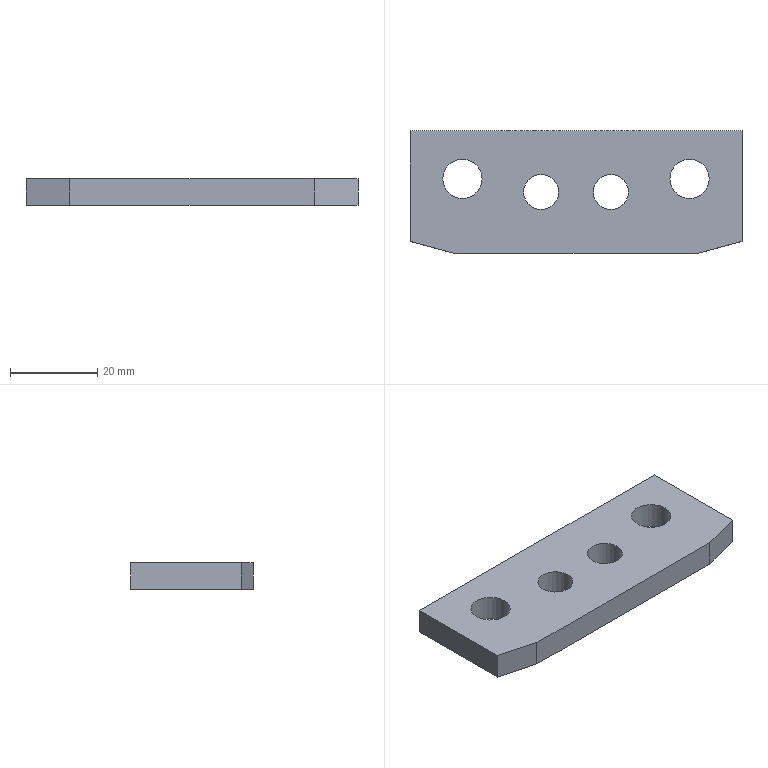Part | STEP file | gslz 2016.10.28-13_id1586_x_t | 1 solid | 12 faces | box 76 x 28 x 6 mm | volume 11241 mm3 | plane 8 | cylinder 4 | commonest cylinder face diameters 8 x2 9 x2
STEP:
#1=CARTESIAN_POINT('',(0.,0.,0.));
#2=DIRECTION('',(0.,0.,1.));
#3=DIRECTION('',(1.,0.,0.));
#4=AXIS2_PLACEMENT_3D('',#1,#2,#3);
#5=CARTESIAN_POINT('',(-1350.002,284.2,6.));
#6=VERTEX_POINT('',#5);
#7=CARTESIAN_POINT('',(-1358.002,284.2,6.));
#8=VERTEX_POINT('',#7);
#9=CARTESIAN_POINT('',(-1354.002,284.2,6.));
#10=DIRECTION('',(0.,0.,1.));
#11=DIRECTION('',(-1.,0.,0.));
#12=AXIS2_PLACEMENT_3D('',#9,#10,#11);
#13=CIRCLE('',#12,4.);
#14=CARTESIAN_POINT('',(-1354.002,284.2,-73.));
#15=DIRECTION('',(0.,0.,1.));
#16=DIRECTION('',(1.,0.,0.));
#17=AXIS2_PLACEMENT_3D('',#14,#15,#16);
#18=CYLINDRICAL_SURFACE('',#17,4.);
#19=CARTESIAN_POINT('',(-3.142,79.));
#20=DIRECTION('',(1.,0.));
#21=VECTOR('',#20,1.);
#22=LINE('',#19,#21);
#23=(GEOMETRIC_REPRESENTATION_CONTEXT(2)PARAMETRIC_REPRESENTATION_CONTEXT()REPRESENTATION_CONTEXT('',''));
#24=DEFINITIONAL_REPRESENTATION('',(#22),#23);
#25=PCURVE('',#18,#24);
#26=CARTESIAN_POINT('',(-1421.002,267.7,6.));
#27=DIRECTION('',(0.,0.,-1.));
#28=DIRECTION('',(-1.,0.,0.));
#29=AXIS2_PLACEMENT_3D('',#26,#27,#28);
#30=PLANE('',#29);
#31=CARTESIAN_POINT('',(-63.,16.5));
#32=CARTESIAN_POINT('',(-63.,9.572));
#33=CARTESIAN_POINT('',(-69.,13.036));
#34=CARTESIAN_POINT('',(-75.,16.5));
#35=CARTESIAN_POINT('',(-69.,19.964));
#36=CARTESIAN_POINT('',(-63.,23.428));
#37=CARTESIAN_POINT('',(-63.,16.5));
#38=(BOUNDED_CURVE()B_SPLINE_CURVE(2,(#31,#32,#33,#34,#35,#36,#37),.UNSPECIFIED.,.T.,.F.)B_SPLINE_CURVE_WITH_KNOTS((1,2,2,2,2,1),(-2.094,0.,2.094,4.189,6.283,8.378),.UNSPECIFIED.)CURVE()GEOMETRIC_REPRESENTATION_ITEM()RATIONAL_B_SPLINE_CURVE((1.,0.5,1.,0.5,1.,0.5,1.))REPRESENTATION_ITEM(''));
#39=(GEOMETRIC_REPRESENTATION_CONTEXT(2)PARAMETRIC_REPRESENTATION_CONTEXT()REPRESENTATION_CONTEXT('',''));
#40=DEFINITIONAL_REPRESENTATION('',(#38),#39);
#41=PCURVE('',#30,#40);
#42=SURFACE_CURVE('',#13,(#25,#41),.PCURVE_S1.);
#43=EDGE_CURVE('',#6,#8,#42,.T.);
#44=ORIENTED_EDGE('',*,*,#43,.F.);
#45=CARTESIAN_POINT('',(-1350.002,284.2,0.));
#46=VERTEX_POINT('',#45);
#47=CARTESIAN_POINT('',(-1350.002,284.2,0.));
#48=CARTESIAN_POINT('',(-1350.002,284.2,6.));
#49=B_SPLINE_CURVE_WITH_KNOTS('',1,(#47,#48),.UNSPECIFIED.,.F.,.F.,(2,2),(73.,79.),.PIECEWISE_BEZIER_KNOTS.);
#50=CARTESIAN_POINT('',(0.,0.));
#51=DIRECTION('',(0.,1.));
#52=VECTOR('',#51,1.);
#53=LINE('',#50,#52);
#54=(GEOMETRIC_REPRESENTATION_CONTEXT(2)PARAMETRIC_REPRESENTATION_CONTEXT()REPRESENTATION_CONTEXT('',''));
#55=DEFINITIONAL_REPRESENTATION('',(#53),#54);
#56=PCURVE('',#18,#55);
#57=CARTESIAN_POINT('',(6.283,0.));
#58=DIRECTION('',(0.,1.));
#59=VECTOR('',#58,1.);
#60=LINE('',#57,#59);
#61=(GEOMETRIC_REPRESENTATION_CONTEXT(2)PARAMETRIC_REPRESENTATION_CONTEXT()REPRESENTATION_CONTEXT('',''));
#62=DEFINITIONAL_REPRESENTATION('',(#60),#61);
#63=PCURVE('',#18,#62);
#64=SEAM_CURVE('',#49,(#56,#63),.PCURVE_S1.);
#65=EDGE_CURVE('',#46,#6,#64,.T.);
#66=ORIENTED_EDGE('',*,*,#65,.F.);
#67=CARTESIAN_POINT('',(-1354.002,284.2,0.));
#68=DIRECTION('',(0.,0.,-1.));
#69=DIRECTION('',(1.,0.,0.));
#70=AXIS2_PLACEMENT_3D('',#67,#68,#69);
#71=CIRCLE('',#70,4.);
#72=CARTESIAN_POINT('',(6.283,73.));
#73=DIRECTION('',(-1.,0.));
#74=VECTOR('',#73,1.);
#75=LINE('',#72,#74);
#76=(GEOMETRIC_REPRESENTATION_CONTEXT(2)PARAMETRIC_REPRESENTATION_CONTEXT()REPRESENTATION_CONTEXT('',''));
#77=DEFINITIONAL_REPRESENTATION('',(#75),#76);
#78=PCURVE('',#18,#77);
#79=CARTESIAN_POINT('',(-1461.002,298.2,0.));
#80=DIRECTION('',(0.,0.,1.));
#81=DIRECTION('',(1.,0.,0.));
#82=AXIS2_PLACEMENT_3D('',#79,#80,#81);
#83=PLANE('',#82);
#84=CARTESIAN_POINT('',(111.,-14.));
#85=CARTESIAN_POINT('',(111.,-20.928));
#86=CARTESIAN_POINT('',(105.,-17.464));
#87=CARTESIAN_POINT('',(99.,-14.));
#88=CARTESIAN_POINT('',(105.,-10.536));
#89=CARTESIAN_POINT('',(111.,-7.072));
#90=CARTESIAN_POINT('',(111.,-14.));
#91=(BOUNDED_CURVE()B_SPLINE_CURVE(2,(#84,#85,#86,#87,#88,#89,#90),.UNSPECIFIED.,.T.,.F.)B_SPLINE_CURVE_WITH_KNOTS((1,2,2,2,2,1),(-2.094,0.,2.094,4.189,6.283,8.378),.UNSPECIFIED.)CURVE()GEOMETRIC_REPRESENTATION_ITEM()RATIONAL_B_SPLINE_CURVE((1.,0.5,1.,0.5,1.,0.5,1.))REPRESENTATION_ITEM(''));
#92=(GEOMETRIC_REPRESENTATION_CONTEXT(2)PARAMETRIC_REPRESENTATION_CONTEXT()REPRESENTATION_CONTEXT('',''));
#93=DEFINITIONAL_REPRESENTATION('',(#91),#92);
#94=PCURVE('',#83,#93);
#95=SURFACE_CURVE('',#71,(#78,#94),.PCURVE_S1.);
#96=EDGE_CURVE('',#46,#46,#95,.T.);
#97=ORIENTED_EDGE('',*,*,#96,.F.);
#98=ORIENTED_EDGE('',*,*,#65,.T.);
#99=CARTESIAN_POINT('',(-1354.002,284.2,6.));
#100=DIRECTION('',(0.,0.,1.));
#101=DIRECTION('',(-1.,0.,0.));
#102=AXIS2_PLACEMENT_3D('',#99,#100,#101);
#103=CIRCLE('',#102,4.);
#104=CARTESIAN_POINT('',(3.142,79.));
#105=DIRECTION('',(1.,0.));
#106=VECTOR('',#105,1.);
#107=LINE('',#104,#106);
#108=(GEOMETRIC_REPRESENTATION_CONTEXT(2)PARAMETRIC_REPRESENTATION_CONTEXT()REPRESENTATION_CONTEXT('',''));
#109=DEFINITIONAL_REPRESENTATION('',(#107),#108);
#110=PCURVE('',#18,#109);
#111=CARTESIAN_POINT('',(-63.,16.5));
#112=CARTESIAN_POINT('',(-63.,9.572));
#113=CARTESIAN_POINT('',(-69.,13.036));
#114=CARTESIAN_POINT('',(-75.,16.5));
#115=CARTESIAN_POINT('',(-69.,19.964));
#116=CARTESIAN_POINT('',(-63.,23.428));
#117=CARTESIAN_POINT('',(-63.,16.5));
#118=(BOUNDED_CURVE()B_SPLINE_CURVE(2,(#111,#112,#113,#114,#115,#116,#117),.UNSPECIFIED.,.T.,.F.)B_SPLINE_CURVE_WITH_KNOTS((1,2,2,2,2,1),(-2.094,0.,2.094,4.189,6.283,8.378),.UNSPECIFIED.)CURVE()GEOMETRIC_REPRESENTATION_ITEM()RATIONAL_B_SPLINE_CURVE((1.,0.5,1.,0.5,1.,0.5,1.))REPRESENTATION_ITEM(''));
#119=(GEOMETRIC_REPRESENTATION_CONTEXT(2)PARAMETRIC_REPRESENTATION_CONTEXT()REPRESENTATION_CONTEXT('',''));
#120=DEFINITIONAL_REPRESENTATION('',(#118),#119);
#121=PCURVE('',#30,#120);
#122=SURFACE_CURVE('',#103,(#110,#121),.PCURVE_S1.);
#123=EDGE_CURVE('',#8,#6,#122,.T.);
#124=ORIENTED_EDGE('',*,*,#123,.F.);
#125=EDGE_LOOP('',(#44,#66,#97,#98,#124));
#126=FACE_BOUND('',#125,.F.);
#127=ADVANCED_FACE('',(#126),#18,.F.);
#128=CARTESIAN_POINT('',(-1342.002,284.2,6.));
#129=VERTEX_POINT('',#128);
#130=CARTESIAN_POINT('',(-1334.002,284.2,6.));
#131=VERTEX_POINT('',#130);
#132=CARTESIAN_POINT('',(-1338.002,284.2,6.));
#133=DIRECTION('',(0.,0.,-1.));
#134=DIRECTION('',(-1.,0.,0.));
#135=AXIS2_PLACEMENT_3D('',#132,#133,#134);
#136=CIRCLE('',#135,4.);
#137=CARTESIAN_POINT('',(-1338.002,284.2,-73.));
#138=DIRECTION('',(0.,0.,1.));
#139=DIRECTION('',(1.,0.,0.));
#140=AXIS2_PLACEMENT_3D('',#137,#138,#139);
#141=CYLINDRICAL_SURFACE('',#140,4.);
#142=CARTESIAN_POINT('',(3.142,79.));
#143=DIRECTION('',(-1.,0.));
#144=VECTOR('',#143,1.);
#145=LINE('',#142,#144);
#146=(GEOMETRIC_REPRESENTATION_CONTEXT(2)PARAMETRIC_REPRESENTATION_CONTEXT()REPRESENTATION_CONTEXT('',''));
#147=DEFINITIONAL_REPRESENTATION('',(#145),#146);
#148=PCURVE('',#141,#147);
#149=CARTESIAN_POINT('',(-83.,16.5));
#150=DIRECTION('',(1.,0.));
#151=AXIS2_PLACEMENT_2D('',#149,#150);
#152=CIRCLE('',#151,4.);
#153=(GEOMETRIC_REPRESENTATION_CONTEXT(2)PARAMETRIC_REPRESENTATION_CONTEXT()REPRESENTATION_CONTEXT('',''));
#154=DEFINITIONAL_REPRESENTATION('',(#152),#153);
#155=PCURVE('',#30,#154);
#156=SURFACE_CURVE('',#136,(#148,#155),.PCURVE_S1.);
#157=EDGE_CURVE('',#129,#131,#156,.T.);
#158=ORIENTED_EDGE('',*,*,#157,.T.);
#159=CARTESIAN_POINT('',(-1334.002,284.2,0.));
#160=VERTEX_POINT('',#159);
#161=CARTESIAN_POINT('',(-1334.002,284.2,0.));
#162=CARTESIAN_POINT('',(-1334.002,284.2,6.));
#163=B_SPLINE_CURVE_WITH_KNOTS('',1,(#161,#162),.UNSPECIFIED.,.F.,.F.,(2,2),(73.,79.),.PIECEWISE_BEZIER_KNOTS.);
#164=CARTESIAN_POINT('',(0.,0.));
#165=DIRECTION('',(0.,1.));
#166=VECTOR('',#165,1.);
#167=LINE('',#164,#166);
#168=(GEOMETRIC_REPRESENTATION_CONTEXT(2)PARAMETRIC_REPRESENTATION_CONTEXT()REPRESENTATION_CONTEXT('',''));
#169=DEFINITIONAL_REPRESENTATION('',(#167),#168);
#170=PCURVE('',#141,#169);
#171=CARTESIAN_POINT('',(6.283,0.));
#172=DIRECTION('',(0.,1.));
#173=VECTOR('',#172,1.);
#174=LINE('',#171,#173);
#175=(GEOMETRIC_REPRESENTATION_CONTEXT(2)PARAMETRIC_REPRESENTATION_CONTEXT()REPRESENTATION_CONTEXT('',''));
#176=DEFINITIONAL_REPRESENTATION('',(#174),#175);
#177=PCURVE('',#141,#176);
#178=SEAM_CURVE('',#163,(#170,#177),.PCURVE_S1.);
#179=EDGE_CURVE('',#160,#131,#178,.T.);
#180=ORIENTED_EDGE('',*,*,#179,.F.);
#181=CARTESIAN_POINT('',(-1338.002,284.2,0.));
#182=DIRECTION('',(0.,0.,1.));
#183=DIRECTION('',(1.,0.,0.));
#184=AXIS2_PLACEMENT_3D('',#181,#182,#183);
#185=CIRCLE('',#184,4.);
#186=CARTESIAN_POINT('',(0.,73.));
#187=DIRECTION('',(1.,0.));
#188=VECTOR('',#187,1.);
#189=LINE('',#186,#188);
#190=(GEOMETRIC_REPRESENTATION_CONTEXT(2)PARAMETRIC_REPRESENTATION_CONTEXT()REPRESENTATION_CONTEXT('',''));
#191=DEFINITIONAL_REPRESENTATION('',(#189),#190);
#192=PCURVE('',#141,#191);
#193=CARTESIAN_POINT('',(123.,-14.));
#194=DIRECTION('',(1.,0.));
#195=AXIS2_PLACEMENT_2D('',#193,#194);
#196=CIRCLE('',#195,4.);
#197=(GEOMETRIC_REPRESENTATION_CONTEXT(2)PARAMETRIC_REPRESENTATION_CONTEXT()REPRESENTATION_CONTEXT('',''));
#198=DEFINITIONAL_REPRESENTATION('',(#196),#197);
#199=PCURVE('',#83,#198);
#200=SURFACE_CURVE('',#185,(#192,#199),.PCURVE_S1.);
#201=EDGE_CURVE('',#160,#160,#200,.T.);
#202=ORIENTED_EDGE('',*,*,#201,.T.);
#203=ORIENTED_EDGE('',*,*,#179,.T.);
#204=CARTESIAN_POINT('',(-1338.002,284.2,6.));
#205=DIRECTION('',(0.,0.,-1.));
#206=DIRECTION('',(-1.,0.,0.));
#207=AXIS2_PLACEMENT_3D('',#204,#205,#206);
#208=CIRCLE('',#207,4.);
#209=CARTESIAN_POINT('',(9.425,79.));
#210=DIRECTION('',(-1.,0.));
#211=VECTOR('',#210,1.);
#212=LINE('',#209,#211);
#213=(GEOMETRIC_REPRESENTATION_CONTEXT(2)PARAMETRIC_REPRESENTATION_CONTEXT()REPRESENTATION_CONTEXT('',''));
#214=DEFINITIONAL_REPRESENTATION('',(#212),#213);
#215=PCURVE('',#141,#214);
#216=CARTESIAN_POINT('',(-83.,16.5));
#217=DIRECTION('',(1.,0.));
#218=AXIS2_PLACEMENT_2D('',#216,#217);
#219=CIRCLE('',#218,4.);
#220=(GEOMETRIC_REPRESENTATION_CONTEXT(2)PARAMETRIC_REPRESENTATION_CONTEXT()REPRESENTATION_CONTEXT('',''));
#221=DEFINITIONAL_REPRESENTATION('',(#219),#220);
#222=PCURVE('',#30,#221);
#223=SURFACE_CURVE('',#208,(#215,#222),.PCURVE_S1.);
#224=EDGE_CURVE('',#131,#129,#223,.T.);
#225=ORIENTED_EDGE('',*,*,#224,.T.);
#226=EDGE_LOOP('',(#158,#180,#202,#203,#225));
#227=FACE_BOUND('',#226,.F.);
#228=ADVANCED_FACE('',(#227),#141,.F.);
#229=CARTESIAN_POINT('',(-1376.502,287.2,6.));
#230=VERTEX_POINT('',#229);
#231=CARTESIAN_POINT('',(-1372.002,287.2,6.));
#232=DIRECTION('',(0.,0.,-1.));
#233=DIRECTION('',(-1.,0.,0.));
#234=AXIS2_PLACEMENT_3D('',#231,#232,#233);
#235=CIRCLE('',#234,4.5);
#236=CARTESIAN_POINT('',(-1372.002,287.2,47.));
#237=DIRECTION('',(0.,0.,-1.));
#238=DIRECTION('',(-1.,0.,0.));
#239=AXIS2_PLACEMENT_3D('',#236,#237,#238);
#240=CYLINDRICAL_SURFACE('',#239,4.5);
#241=CARTESIAN_POINT('',(0.,41.));
#242=DIRECTION('',(1.,0.));
#243=VECTOR('',#242,1.);
#244=LINE('',#241,#243);
#245=(GEOMETRIC_REPRESENTATION_CONTEXT(2)PARAMETRIC_REPRESENTATION_CONTEXT()REPRESENTATION_CONTEXT('',''));
#246=DEFINITIONAL_REPRESENTATION('',(#244),#245);
#247=PCURVE('',#240,#246);
#248=CARTESIAN_POINT('',(-49.,19.5));
#249=DIRECTION('',(1.,0.));
#250=AXIS2_PLACEMENT_2D('',#248,#249);
#251=CIRCLE('',#250,4.5);
#252=(GEOMETRIC_REPRESENTATION_CONTEXT(2)PARAMETRIC_REPRESENTATION_CONTEXT()REPRESENTATION_CONTEXT('',''));
#253=DEFINITIONAL_REPRESENTATION('',(#251),#252);
#254=PCURVE('',#30,#253);
#255=SURFACE_CURVE('',#235,(#247,#254),.PCURVE_S1.);
#256=EDGE_CURVE('',#230,#230,#255,.T.);
#257=ORIENTED_EDGE('',*,*,#256,.T.);
#258=CARTESIAN_POINT('',(-1376.502,287.2,0.));
#259=VERTEX_POINT('',#258);
#260=CARTESIAN_POINT('',(-1376.502,287.2,6.));
#261=CARTESIAN_POINT('',(-1376.502,287.2,0.));
#262=B_SPLINE_CURVE_WITH_KNOTS('',1,(#260,#261),.UNSPECIFIED.,.F.,.F.,(2,2),(41.,47.),.PIECEWISE_BEZIER_KNOTS.);
#263=CARTESIAN_POINT('',(6.283,0.));
#264=DIRECTION('',(0.,1.));
#265=VECTOR('',#264,1.);
#266=LINE('',#263,#265);
#267=(GEOMETRIC_REPRESENTATION_CONTEXT(2)PARAMETRIC_REPRESENTATION_CONTEXT()REPRESENTATION_CONTEXT('',''));
#268=DEFINITIONAL_REPRESENTATION('',(#266),#267);
#269=PCURVE('',#240,#268);
#270=CARTESIAN_POINT('',(0.,0.));
#271=DIRECTION('',(0.,1.));
#272=VECTOR('',#271,1.);
#273=LINE('',#270,#272);
#274=(GEOMETRIC_REPRESENTATION_CONTEXT(2)PARAMETRIC_REPRESENTATION_CONTEXT()REPRESENTATION_CONTEXT('',''));
#275=DEFINITIONAL_REPRESENTATION('',(#273),#274);
#276=PCURVE('',#240,#275);
#277=SEAM_CURVE('',#262,(#269,#276),.PCURVE_S1.);
#278=EDGE_CURVE('',#230,#259,#277,.T.);
#279=ORIENTED_EDGE('',*,*,#278,.T.);
#280=CARTESIAN_POINT('',(-1367.502,287.2,0.));
#281=VERTEX_POINT('',#280);
#282=CARTESIAN_POINT('',(-1372.002,287.2,0.));
#283=DIRECTION('',(0.,0.,1.));
#284=DIRECTION('',(1.,0.,0.));
#285=AXIS2_PLACEMENT_3D('',#282,#283,#284);
#286=CIRCLE('',#285,4.5);
#287=CARTESIAN_POINT('',(9.425,47.));
#288=DIRECTION('',(-1.,0.));
#289=VECTOR('',#288,1.);
#290=LINE('',#287,#289);
#291=(GEOMETRIC_REPRESENTATION_CONTEXT(2)PARAMETRIC_REPRESENTATION_CONTEXT()REPRESENTATION_CONTEXT('',''));
#292=DEFINITIONAL_REPRESENTATION('',(#290),#291);
#293=PCURVE('',#240,#292);
#294=CARTESIAN_POINT('',(89.,-11.));
#295=DIRECTION('',(1.,0.));
#296=AXIS2_PLACEMENT_2D('',#294,#295);
#297=CIRCLE('',#296,4.5);
#298=(GEOMETRIC_REPRESENTATION_CONTEXT(2)PARAMETRIC_REPRESENTATION_CONTEXT()REPRESENTATION_CONTEXT('',''));
#299=DEFINITIONAL_REPRESENTATION('',(#297),#298);
#300=PCURVE('',#83,#299);
#301=SURFACE_CURVE('',#286,(#293,#300),.PCURVE_S1.);
#302=EDGE_CURVE('',#259,#281,#301,.T.);
#303=ORIENTED_EDGE('',*,*,#302,.T.);
#304=CARTESIAN_POINT('',(-1372.002,287.2,0.));
#305=DIRECTION('',(0.,0.,1.));
#306=DIRECTION('',(1.,0.,0.));
#307=AXIS2_PLACEMENT_3D('',#304,#305,#306);
#308=CIRCLE('',#307,4.5);
#309=CARTESIAN_POINT('',(3.142,47.));
#310=DIRECTION('',(-1.,0.));
#311=VECTOR('',#310,1.);
#312=LINE('',#309,#311);
#313=(GEOMETRIC_REPRESENTATION_CONTEXT(2)PARAMETRIC_REPRESENTATION_CONTEXT()REPRESENTATION_CONTEXT('',''));
#314=DEFINITIONAL_REPRESENTATION('',(#312),#313);
#315=PCURVE('',#240,#314);
#316=CARTESIAN_POINT('',(89.,-11.));
#317=DIRECTION('',(1.,0.));
#318=AXIS2_PLACEMENT_2D('',#316,#317);
#319=CIRCLE('',#318,4.5);
#320=(GEOMETRIC_REPRESENTATION_CONTEXT(2)PARAMETRIC_REPRESENTATION_CONTEXT()REPRESENTATION_CONTEXT('',''));
#321=DEFINITIONAL_REPRESENTATION('',(#319),#320);
#322=PCURVE('',#83,#321);
#323=SURFACE_CURVE('',#308,(#315,#322),.PCURVE_S1.);
#324=EDGE_CURVE('',#281,#259,#323,.T.);
#325=ORIENTED_EDGE('',*,*,#324,.T.);
#326=ORIENTED_EDGE('',*,*,#278,.F.);
#327=EDGE_LOOP('',(#257,#279,#303,#325,#326));
#328=FACE_BOUND('',#327,.F.);
#329=ADVANCED_FACE('',(#328),#240,.F.);
#330=CARTESIAN_POINT('',(-1318.001,270.2,0.));
#331=VERTEX_POINT('',#330);
#332=CARTESIAN_POINT('',(-1318.001,270.2,6.));
#333=VERTEX_POINT('',#332);
#334=CARTESIAN_POINT('',(-1318.001,270.2,8.));
#335=DIRECTION('',(0.,0.,1.));
#336=VECTOR('',#335,1.);
#337=LINE('',#334,#336);
#338=CARTESIAN_POINT('',(-1451.,270.2,8.));
#339=DIRECTION('',(0.,1.,0.));
#340=DIRECTION('',(0.,0.,1.));
#341=AXIS2_PLACEMENT_3D('',#338,#339,#340);
#342=PLANE('',#341);
#343=CARTESIAN_POINT('',(0.,132.999));
#344=DIRECTION('',(1.,0.));
#345=VECTOR('',#344,1.);
#346=LINE('',#343,#345);
#347=(GEOMETRIC_REPRESENTATION_CONTEXT(2)PARAMETRIC_REPRESENTATION_CONTEXT()REPRESENTATION_CONTEXT('',''));
#348=DEFINITIONAL_REPRESENTATION('',(#346),#347);
#349=PCURVE('',#342,#348);
#350=CARTESIAN_POINT('',(-1318.001,270.2,8.));
#351=DIRECTION('',(-0.2588,0.9659,0.));
#352=DIRECTION('',(-0.9659,-0.2588,0.));
#353=AXIS2_PLACEMENT_3D('',#350,#351,#352);
#354=PLANE('',#353);
#355=CARTESIAN_POINT('',(0.,0.));
#356=DIRECTION('',(0.,1.));
#357=VECTOR('',#356,1.);
#358=LINE('',#355,#357);
#359=(GEOMETRIC_REPRESENTATION_CONTEXT(2)PARAMETRIC_REPRESENTATION_CONTEXT()REPRESENTATION_CONTEXT('',''));
#360=DEFINITIONAL_REPRESENTATION('',(#358),#359);
#361=PCURVE('',#354,#360);
#362=SURFACE_CURVE('',#337,(#349,#361),.PCURVE_S1.);
#363=EDGE_CURVE('',#331,#333,#362,.T.);
#364=ORIENTED_EDGE('',*,*,#363,.T.);
#365=CARTESIAN_POINT('',(-1374.,270.2,6.));
#366=VERTEX_POINT('',#365);
#367=CARTESIAN_POINT('',(-1451.,270.2,6.));
#368=DIRECTION('',(-1.,0.,0.));
#369=VECTOR('',#368,1.);
#370=LINE('',#367,#369);
#371=CARTESIAN_POINT('',(-2.,0.));
#372=DIRECTION('',(0.,-1.));
#373=VECTOR('',#372,1.);
#374=LINE('',#371,#373);
#375=(GEOMETRIC_REPRESENTATION_CONTEXT(2)PARAMETRIC_REPRESENTATION_CONTEXT()REPRESENTATION_CONTEXT('',''));
#376=DEFINITIONAL_REPRESENTATION('',(#374),#375);
#377=PCURVE('',#342,#376);
#378=CARTESIAN_POINT('',(29.998,2.5));
#379=DIRECTION('',(1.,0.));
#380=VECTOR('',#379,1.);
#381=LINE('',#378,#380);
#382=(GEOMETRIC_REPRESENTATION_CONTEXT(2)PARAMETRIC_REPRESENTATION_CONTEXT()REPRESENTATION_CONTEXT('',''));
#383=DEFINITIONAL_REPRESENTATION('',(#381),#382);
#384=PCURVE('',#30,#383);
#385=SURFACE_CURVE('',#370,(#377,#384),.PCURVE_S1.);
#386=EDGE_CURVE('',#333,#366,#385,.T.);
#387=ORIENTED_EDGE('',*,*,#386,.T.);
#388=CARTESIAN_POINT('',(-1374.,270.2,0.));
#389=VERTEX_POINT('',#388);
#390=CARTESIAN_POINT('',(-1374.,270.2,8.));
#391=DIRECTION('',(0.,0.,1.));
#392=VECTOR('',#391,1.);
#393=LINE('',#390,#392);
#394=CARTESIAN_POINT('',(0.,77.));
#395=DIRECTION('',(1.,0.));
#396=VECTOR('',#395,1.);
#397=LINE('',#394,#396);
#398=(GEOMETRIC_REPRESENTATION_CONTEXT(2)PARAMETRIC_REPRESENTATION_CONTEXT()REPRESENTATION_CONTEXT('',''));
#399=DEFINITIONAL_REPRESENTATION('',(#397),#398);
#400=PCURVE('',#342,#399);
#401=CARTESIAN_POINT('',(-1384.002,272.88,8.));
#402=DIRECTION('',(0.2588,0.9659,0.));
#403=DIRECTION('',(-0.9659,0.2588,0.));
#404=AXIS2_PLACEMENT_3D('',#401,#402,#403);
#405=PLANE('',#404);
#406=CARTESIAN_POINT('',(-10.355,0.));
#407=DIRECTION('',(0.,1.));
#408=VECTOR('',#407,1.);
#409=LINE('',#406,#408);
#410=(GEOMETRIC_REPRESENTATION_CONTEXT(2)PARAMETRIC_REPRESENTATION_CONTEXT()REPRESENTATION_CONTEXT('',''));
#411=DEFINITIONAL_REPRESENTATION('',(#409),#410);
#412=PCURVE('',#405,#411);
#413=SURFACE_CURVE('',#393,(#400,#412),.PCURVE_S1.);
#414=EDGE_CURVE('',#389,#366,#413,.T.);
#415=ORIENTED_EDGE('',*,*,#414,.F.);
#416=CARTESIAN_POINT('',(-1451.,270.2,0.));
#417=DIRECTION('',(1.,0.,0.));
#418=VECTOR('',#417,1.);
#419=LINE('',#416,#418);
#420=CARTESIAN_POINT('',(-8.,0.));
#421=DIRECTION('',(0.,1.));
#422=VECTOR('',#421,1.);
#423=LINE('',#420,#422);
#424=(GEOMETRIC_REPRESENTATION_CONTEXT(2)PARAMETRIC_REPRESENTATION_CONTEXT()REPRESENTATION_CONTEXT('',''));
#425=DEFINITIONAL_REPRESENTATION('',(#423),#424);
#426=PCURVE('',#342,#425);
#427=CARTESIAN_POINT('',(10.002,-28.));
#428=DIRECTION('',(1.,0.));
#429=VECTOR('',#428,1.);
#430=LINE('',#427,#429);
#431=(GEOMETRIC_REPRESENTATION_CONTEXT(2)PARAMETRIC_REPRESENTATION_CONTEXT()REPRESENTATION_CONTEXT('',''));
#432=DEFINITIONAL_REPRESENTATION('',(#430),#431);
#433=PCURVE('',#83,#432);
#434=SURFACE_CURVE('',#419,(#426,#433),.PCURVE_S1.);
#435=EDGE_CURVE('',#389,#331,#434,.T.);
#436=ORIENTED_EDGE('',*,*,#435,.T.);
#437=EDGE_LOOP('',(#364,#387,#415,#436));
#438=FACE_BOUND('',#437,.T.);
#439=ADVANCED_FACE('',(#438),#342,.F.);
#440=CARTESIAN_POINT('',(-1308.002,272.879,6.));
#441=VERTEX_POINT('',#440);
#442=CARTESIAN_POINT('',(-1308.002,272.879,0.));
#443=VERTEX_POINT('',#442);
#444=CARTESIAN_POINT('',(-1308.002,272.879,8.));
#445=DIRECTION('',(0.,0.,-1.));
#446=VECTOR('',#445,1.);
#447=LINE('',#444,#446);
#448=CARTESIAN_POINT('',(-10.352,0.));
#449=DIRECTION('',(0.,-1.));
#450=VECTOR('',#449,1.);
#451=LINE('',#448,#450);
#452=(GEOMETRIC_REPRESENTATION_CONTEXT(2)PARAMETRIC_REPRESENTATION_CONTEXT()REPRESENTATION_CONTEXT('',''));
#453=DEFINITIONAL_REPRESENTATION('',(#451),#452);
#454=PCURVE('',#354,#453);
#455=CARTESIAN_POINT('',(-1308.002,265.2,16.));
#456=DIRECTION('',(-1.,0.,0.));
#457=DIRECTION('',(0.,0.,1.));
#458=AXIS2_PLACEMENT_3D('',#455,#456,#457);
#459=PLANE('',#458);
#460=CARTESIAN_POINT('',(-8.,7.679));
#461=DIRECTION('',(-1.,0.));
#462=VECTOR('',#461,1.);
#463=LINE('',#460,#462);
#464=(GEOMETRIC_REPRESENTATION_CONTEXT(2)PARAMETRIC_REPRESENTATION_CONTEXT()REPRESENTATION_CONTEXT('',''));
#465=DEFINITIONAL_REPRESENTATION('',(#463),#464);
#466=PCURVE('',#459,#465);
#467=SURFACE_CURVE('',#447,(#454,#466),.PCURVE_S1.);
#468=EDGE_CURVE('',#441,#443,#467,.T.);
#469=ORIENTED_EDGE('',*,*,#468,.F.);
#470=CARTESIAN_POINT('',(-1318.001,270.2,6.));
#471=DIRECTION('',(-0.9659,-0.2588,0.));
#472=VECTOR('',#471,1.);
#473=LINE('',#470,#472);
#474=CARTESIAN_POINT('',(0.,-2.));
#475=DIRECTION('',(1.,0.));
#476=VECTOR('',#475,1.);
#477=LINE('',#474,#476);
#478=(GEOMETRIC_REPRESENTATION_CONTEXT(2)PARAMETRIC_REPRESENTATION_CONTEXT()REPRESENTATION_CONTEXT('',''));
#479=DEFINITIONAL_REPRESENTATION('',(#477),#478);
#480=PCURVE('',#354,#479);
#481=CARTESIAN_POINT('',(-103.001,2.5));
#482=DIRECTION('',(0.9659,-0.2588));
#483=VECTOR('',#482,1.);
#484=LINE('',#481,#483);
#485=(GEOMETRIC_REPRESENTATION_CONTEXT(2)PARAMETRIC_REPRESENTATION_CONTEXT()REPRESENTATION_CONTEXT('',''));
#486=DEFINITIONAL_REPRESENTATION('',(#484),#485);
#487=PCURVE('',#30,#486);
#488=SURFACE_CURVE('',#473,(#480,#487),.PCURVE_S1.);
#489=EDGE_CURVE('',#441,#333,#488,.T.);
#490=ORIENTED_EDGE('',*,*,#489,.T.);
#491=ORIENTED_EDGE('',*,*,#363,.F.);
#492=CARTESIAN_POINT('',(-1318.001,270.2,0.));
#493=DIRECTION('',(0.9659,0.2588,0.));
#494=VECTOR('',#493,1.);
#495=LINE('',#492,#494);
#496=CARTESIAN_POINT('',(0.,-8.));
#497=DIRECTION('',(-1.,0.));
#498=VECTOR('',#497,1.);
#499=LINE('',#496,#498);
#500=(GEOMETRIC_REPRESENTATION_CONTEXT(2)PARAMETRIC_REPRESENTATION_CONTEXT()REPRESENTATION_CONTEXT('',''));
#501=DEFINITIONAL_REPRESENTATION('',(#499),#500);
#502=PCURVE('',#354,#501);
#503=CARTESIAN_POINT('',(143.001,-28.));
#504=DIRECTION('',(0.9659,0.2588));
#505=VECTOR('',#504,1.);
#506=LINE('',#503,#505);
#507=(GEOMETRIC_REPRESENTATION_CONTEXT(2)PARAMETRIC_REPRESENTATION_CONTEXT()REPRESENTATION_CONTEXT('',''));
#508=DEFINITIONAL_REPRESENTATION('',(#506),#507);
#509=PCURVE('',#83,#508);
#510=SURFACE_CURVE('',#495,(#502,#509),.PCURVE_S1.);
#511=EDGE_CURVE('',#331,#443,#510,.T.);
#512=ORIENTED_EDGE('',*,*,#511,.T.);
#513=EDGE_LOOP('',(#469,#490,#491,#512));
#514=FACE_BOUND('',#513,.T.);
#515=ADVANCED_FACE('',(#514),#354,.F.);
#516=CARTESIAN_POINT('',(-1308.002,298.2,6.));
#517=VERTEX_POINT('',#516);
#518=CARTESIAN_POINT('',(-1308.002,298.2,0.));
#519=VERTEX_POINT('',#518);
#520=CARTESIAN_POINT('',(-1308.002,298.2,16.));
#521=DIRECTION('',(0.,0.,-1.));
#522=VECTOR('',#521,1.);
#523=LINE('',#520,#522);
#524=CARTESIAN_POINT('',(0.,33.));
#525=DIRECTION('',(-1.,0.));
#526=VECTOR('',#525,1.);
#527=LINE('',#524,#526);
#528=(GEOMETRIC_REPRESENTATION_CONTEXT(2)PARAMETRIC_REPRESENTATION_CONTEXT()REPRESENTATION_CONTEXT('',''));
#529=DEFINITIONAL_REPRESENTATION('',(#527),#528);
#530=PCURVE('',#459,#529);
#531=CARTESIAN_POINT('',(-1381.002,298.2,16.));
#532=DIRECTION('',(0.,-1.,0.));
#533=DIRECTION('',(0.,0.,-1.));
#534=AXIS2_PLACEMENT_3D('',#531,#532,#533);
#535=PLANE('',#534);
#536=CARTESIAN_POINT('',(0.,73.));
#537=DIRECTION('',(1.,0.));
#538=VECTOR('',#537,1.);
#539=LINE('',#536,#538);
#540=(GEOMETRIC_REPRESENTATION_CONTEXT(2)PARAMETRIC_REPRESENTATION_CONTEXT()REPRESENTATION_CONTEXT('',''));
#541=DEFINITIONAL_REPRESENTATION('',(#539),#540);
#542=PCURVE('',#535,#541);
#543=SURFACE_CURVE('',#523,(#530,#542),.PCURVE_S1.);
#544=EDGE_CURVE('',#517,#519,#543,.T.);
#545=ORIENTED_EDGE('',*,*,#544,.F.);
#546=CARTESIAN_POINT('',(-1308.002,265.2,6.));
#547=DIRECTION('',(0.,-1.,0.));
#548=VECTOR('',#547,1.);
#549=LINE('',#546,#548);
#550=CARTESIAN_POINT('',(-10.,0.));
#551=DIRECTION('',(0.,-1.));
#552=VECTOR('',#551,1.);
#553=LINE('',#550,#552);
#554=(GEOMETRIC_REPRESENTATION_CONTEXT(2)PARAMETRIC_REPRESENTATION_CONTEXT()REPRESENTATION_CONTEXT('',''));
#555=DEFINITIONAL_REPRESENTATION('',(#553),#554);
#556=PCURVE('',#459,#555);
#557=CARTESIAN_POINT('',(-113.,-2.5));
#558=DIRECTION('',(0.,-1.));
#559=VECTOR('',#558,1.);
#560=LINE('',#557,#559);
#561=(GEOMETRIC_REPRESENTATION_CONTEXT(2)PARAMETRIC_REPRESENTATION_CONTEXT()REPRESENTATION_CONTEXT('',''));
#562=DEFINITIONAL_REPRESENTATION('',(#560),#561);
#563=PCURVE('',#30,#562);
#564=SURFACE_CURVE('',#549,(#556,#563),.PCURVE_S1.);
#565=EDGE_CURVE('',#517,#441,#564,.T.);
#566=ORIENTED_EDGE('',*,*,#565,.T.);
#567=ORIENTED_EDGE('',*,*,#468,.T.);
#568=CARTESIAN_POINT('',(-1308.002,265.2,0.));
#569=DIRECTION('',(0.,1.,0.));
#570=VECTOR('',#569,1.);
#571=LINE('',#568,#570);
#572=CARTESIAN_POINT('',(-16.,0.));
#573=DIRECTION('',(0.,1.));
#574=VECTOR('',#573,1.);
#575=LINE('',#572,#574);
#576=(GEOMETRIC_REPRESENTATION_CONTEXT(2)PARAMETRIC_REPRESENTATION_CONTEXT()REPRESENTATION_CONTEXT('',''));
#577=DEFINITIONAL_REPRESENTATION('',(#575),#576);
#578=PCURVE('',#459,#577);
#579=CARTESIAN_POINT('',(153.,-33.));
#580=DIRECTION('',(0.,1.));
#581=VECTOR('',#580,1.);
#582=LINE('',#579,#581);
#583=(GEOMETRIC_REPRESENTATION_CONTEXT(2)PARAMETRIC_REPRESENTATION_CONTEXT()REPRESENTATION_CONTEXT('',''));
#584=DEFINITIONAL_REPRESENTATION('',(#582),#583);
#585=PCURVE('',#83,#584);
#586=SURFACE_CURVE('',#571,(#578,#585),.PCURVE_S1.);
#587=EDGE_CURVE('',#443,#519,#586,.T.);
#588=ORIENTED_EDGE('',*,*,#587,.T.);
#589=EDGE_LOOP('',(#545,#566,#567,#588));
#590=FACE_BOUND('',#589,.T.);
#591=ADVANCED_FACE('',(#590),#459,.F.);
#592=CARTESIAN_POINT('',(-1384.002,298.2,6.));
#593=VERTEX_POINT('',#592);
#594=CARTESIAN_POINT('',(-1384.002,298.2,0.));
#595=VERTEX_POINT('',#594);
#596=CARTESIAN_POINT('',(-1384.002,298.2,16.));
#597=DIRECTION('',(0.,0.,-1.));
#598=VECTOR('',#597,1.);
#599=LINE('',#596,#598);
#600=CARTESIAN_POINT('',(0.,-3.));
#601=DIRECTION('',(1.,0.));
#602=VECTOR('',#601,1.);
#603=LINE('',#600,#602);
#604=(GEOMETRIC_REPRESENTATION_CONTEXT(2)PARAMETRIC_REPRESENTATION_CONTEXT()REPRESENTATION_CONTEXT('',''));
#605=DEFINITIONAL_REPRESENTATION('',(#603),#604);
#606=PCURVE('',#535,#605);
#607=CARTESIAN_POINT('',(-1384.002,298.2,16.));
#608=DIRECTION('',(1.,0.,0.));
#609=DIRECTION('',(0.,0.,-1.));
#610=AXIS2_PLACEMENT_3D('',#607,#608,#609);
#611=PLANE('',#610);
#612=CARTESIAN_POINT('',(0.,0.));
#613=DIRECTION('',(1.,0.));
#614=VECTOR('',#613,1.);
#615=LINE('',#612,#614);
#616=(GEOMETRIC_REPRESENTATION_CONTEXT(2)PARAMETRIC_REPRESENTATION_CONTEXT()REPRESENTATION_CONTEXT('',''));
#617=DEFINITIONAL_REPRESENTATION('',(#615),#616);
#618=PCURVE('',#611,#617);
#619=SURFACE_CURVE('',#599,(#606,#618),.PCURVE_S1.);
#620=EDGE_CURVE('',#593,#595,#619,.T.);
#621=ORIENTED_EDGE('',*,*,#620,.F.);
#622=CARTESIAN_POINT('',(-1381.002,298.2,6.));
#623=DIRECTION('',(1.,0.,0.));
#624=VECTOR('',#623,1.);
#625=LINE('',#622,#624);
#626=CARTESIAN_POINT('',(10.,0.));
#627=DIRECTION('',(0.,1.));
#628=VECTOR('',#627,1.);
#629=LINE('',#626,#628);
#630=(GEOMETRIC_REPRESENTATION_CONTEXT(2)PARAMETRIC_REPRESENTATION_CONTEXT()REPRESENTATION_CONTEXT('',''));
#631=DEFINITIONAL_REPRESENTATION('',(#629),#630);
#632=PCURVE('',#535,#631);
#633=CARTESIAN_POINT('',(-40.,30.5));
#634=DIRECTION('',(-1.,0.));
#635=VECTOR('',#634,1.);
#636=LINE('',#633,#635);
#637=(GEOMETRIC_REPRESENTATION_CONTEXT(2)PARAMETRIC_REPRESENTATION_CONTEXT()REPRESENTATION_CONTEXT('',''));
#638=DEFINITIONAL_REPRESENTATION('',(#636),#637);
#639=PCURVE('',#30,#638);
#640=SURFACE_CURVE('',#625,(#632,#639),.PCURVE_S1.);
#641=EDGE_CURVE('',#593,#517,#640,.T.);
#642=ORIENTED_EDGE('',*,*,#641,.T.);
#643=ORIENTED_EDGE('',*,*,#544,.T.);
#644=CARTESIAN_POINT('',(-1381.002,298.2,0.));
#645=DIRECTION('',(-1.,0.,0.));
#646=VECTOR('',#645,1.);
#647=LINE('',#644,#646);
#648=CARTESIAN_POINT('',(16.,0.));
#649=DIRECTION('',(0.,-1.));
#650=VECTOR('',#649,1.);
#651=LINE('',#648,#650);
#652=(GEOMETRIC_REPRESENTATION_CONTEXT(2)PARAMETRIC_REPRESENTATION_CONTEXT()REPRESENTATION_CONTEXT('',''));
#653=DEFINITIONAL_REPRESENTATION('',(#651),#652);
#654=PCURVE('',#535,#653);
#655=CARTESIAN_POINT('',(80.,0.));
#656=DIRECTION('',(-1.,0.));
#657=VECTOR('',#656,1.);
#658=LINE('',#655,#657);
#659=(GEOMETRIC_REPRESENTATION_CONTEXT(2)PARAMETRIC_REPRESENTATION_CONTEXT()REPRESENTATION_CONTEXT('',''));
#660=DEFINITIONAL_REPRESENTATION('',(#658),#659);
#661=PCURVE('',#83,#660);
#662=SURFACE_CURVE('',#647,(#654,#661),.PCURVE_S1.);
#663=EDGE_CURVE('',#519,#595,#662,.T.);
#664=ORIENTED_EDGE('',*,*,#663,.T.);
#665=EDGE_LOOP('',(#621,#642,#643,#664));
#666=FACE_BOUND('',#665,.T.);
#667=ADVANCED_FACE('',(#666),#535,.F.);
#668=CARTESIAN_POINT('',(-1384.002,272.88,6.));
#669=VERTEX_POINT('',#668);
#670=CARTESIAN_POINT('',(-1384.002,272.88,0.));
#671=VERTEX_POINT('',#670);
#672=CARTESIAN_POINT('',(-1384.002,272.88,8.));
#673=DIRECTION('',(0.,0.,-1.));
#674=VECTOR('',#673,1.);
#675=LINE('',#672,#674);
#676=CARTESIAN_POINT('',(8.,-25.32));
#677=DIRECTION('',(1.,0.));
#678=VECTOR('',#677,1.);
#679=LINE('',#676,#678);
#680=(GEOMETRIC_REPRESENTATION_CONTEXT(2)PARAMETRIC_REPRESENTATION_CONTEXT()REPRESENTATION_CONTEXT('',''));
#681=DEFINITIONAL_REPRESENTATION('',(#679),#680);
#682=PCURVE('',#611,#681);
#683=CARTESIAN_POINT('',(0.,0.));
#684=DIRECTION('',(0.,-1.));
#685=VECTOR('',#684,1.);
#686=LINE('',#683,#685);
#687=(GEOMETRIC_REPRESENTATION_CONTEXT(2)PARAMETRIC_REPRESENTATION_CONTEXT()REPRESENTATION_CONTEXT('',''));
#688=DEFINITIONAL_REPRESENTATION('',(#686),#687);
#689=PCURVE('',#405,#688);
#690=SURFACE_CURVE('',#675,(#682,#689),.PCURVE_S1.);
#691=EDGE_CURVE('',#669,#671,#690,.T.);
#692=ORIENTED_EDGE('',*,*,#691,.F.);
#693=CARTESIAN_POINT('',(-1384.002,298.2,6.));
#694=DIRECTION('',(0.,1.,0.));
#695=VECTOR('',#694,1.);
#696=LINE('',#693,#695);
#697=CARTESIAN_POINT('',(10.,0.));
#698=DIRECTION('',(0.,1.));
#699=VECTOR('',#698,1.);
#700=LINE('',#697,#699);
#701=(GEOMETRIC_REPRESENTATION_CONTEXT(2)PARAMETRIC_REPRESENTATION_CONTEXT()REPRESENTATION_CONTEXT('',''));
#702=DEFINITIONAL_REPRESENTATION('',(#700),#701);
#703=PCURVE('',#611,#702);
#704=CARTESIAN_POINT('',(-37.,30.5));
#705=DIRECTION('',(0.,1.));
#706=VECTOR('',#705,1.);
#707=LINE('',#704,#706);
#708=(GEOMETRIC_REPRESENTATION_CONTEXT(2)PARAMETRIC_REPRESENTATION_CONTEXT()REPRESENTATION_CONTEXT('',''));
#709=DEFINITIONAL_REPRESENTATION('',(#707),#708);
#710=PCURVE('',#30,#709);
#711=SURFACE_CURVE('',#696,(#703,#710),.PCURVE_S1.);
#712=EDGE_CURVE('',#669,#593,#711,.T.);
#713=ORIENTED_EDGE('',*,*,#712,.T.);
#714=ORIENTED_EDGE('',*,*,#620,.T.);
#715=CARTESIAN_POINT('',(-1384.002,298.2,0.));
#716=DIRECTION('',(0.,-1.,0.));
#717=VECTOR('',#716,1.);
#718=LINE('',#715,#717);
#719=CARTESIAN_POINT('',(16.,0.));
#720=DIRECTION('',(0.,-1.));
#721=VECTOR('',#720,1.);
#722=LINE('',#719,#721);
#723=(GEOMETRIC_REPRESENTATION_CONTEXT(2)PARAMETRIC_REPRESENTATION_CONTEXT()REPRESENTATION_CONTEXT('',''));
#724=DEFINITIONAL_REPRESENTATION('',(#722),#723);
#725=PCURVE('',#611,#724);
#726=CARTESIAN_POINT('',(77.,0.));
#727=DIRECTION('',(0.,-1.));
#728=VECTOR('',#727,1.);
#729=LINE('',#726,#728);
#730=(GEOMETRIC_REPRESENTATION_CONTEXT(2)PARAMETRIC_REPRESENTATION_CONTEXT()REPRESENTATION_CONTEXT('',''));
#731=DEFINITIONAL_REPRESENTATION('',(#729),#730);
#732=PCURVE('',#83,#731);
#733=SURFACE_CURVE('',#718,(#725,#732),.PCURVE_S1.);
#734=EDGE_CURVE('',#595,#671,#733,.T.);
#735=ORIENTED_EDGE('',*,*,#734,.T.);
#736=EDGE_LOOP('',(#692,#713,#714,#735));
#737=FACE_BOUND('',#736,.T.);
#738=ADVANCED_FACE('',(#737),#611,.F.);
#739=ORIENTED_EDGE('',*,*,#414,.T.);
#740=CARTESIAN_POINT('',(-1384.002,272.88,6.));
#741=DIRECTION('',(-0.9659,0.2588,0.));
#742=VECTOR('',#741,1.);
#743=LINE('',#740,#742);
#744=CARTESIAN_POINT('',(0.,-2.));
#745=DIRECTION('',(1.,0.));
#746=VECTOR('',#745,1.);
#747=LINE('',#744,#746);
#748=(GEOMETRIC_REPRESENTATION_CONTEXT(2)PARAMETRIC_REPRESENTATION_CONTEXT()REPRESENTATION_CONTEXT('',''));
#749=DEFINITIONAL_REPRESENTATION('',(#747),#748);
#750=PCURVE('',#405,#749);
#751=CARTESIAN_POINT('',(-37.,5.18));
#752=DIRECTION('',(0.9659,0.2588));
#753=VECTOR('',#752,1.);
#754=LINE('',#751,#753);
#755=(GEOMETRIC_REPRESENTATION_CONTEXT(2)PARAMETRIC_REPRESENTATION_CONTEXT()REPRESENTATION_CONTEXT('',''));
#756=DEFINITIONAL_REPRESENTATION('',(#754),#755);
#757=PCURVE('',#30,#756);
#758=SURFACE_CURVE('',#743,(#750,#757),.PCURVE_S1.);
#759=EDGE_CURVE('',#366,#669,#758,.T.);
#760=ORIENTED_EDGE('',*,*,#759,.T.);
#761=ORIENTED_EDGE('',*,*,#691,.T.);
#762=CARTESIAN_POINT('',(-1384.002,272.88,0.));
#763=DIRECTION('',(0.9659,-0.2588,0.));
#764=VECTOR('',#763,1.);
#765=LINE('',#762,#764);
#766=CARTESIAN_POINT('',(0.,-8.));
#767=DIRECTION('',(-1.,0.));
#768=VECTOR('',#767,1.);
#769=LINE('',#766,#768);
#770=(GEOMETRIC_REPRESENTATION_CONTEXT(2)PARAMETRIC_REPRESENTATION_CONTEXT()REPRESENTATION_CONTEXT('',''));
#771=DEFINITIONAL_REPRESENTATION('',(#769),#770);
#772=PCURVE('',#405,#771);
#773=CARTESIAN_POINT('',(77.,-25.32));
#774=DIRECTION('',(0.9659,-0.2588));
#775=VECTOR('',#774,1.);
#776=LINE('',#773,#775);
#777=(GEOMETRIC_REPRESENTATION_CONTEXT(2)PARAMETRIC_REPRESENTATION_CONTEXT()REPRESENTATION_CONTEXT('',''));
#778=DEFINITIONAL_REPRESENTATION('',(#776),#777);
#779=PCURVE('',#83,#778);
#780=SURFACE_CURVE('',#765,(#772,#779),.PCURVE_S1.);
#781=EDGE_CURVE('',#671,#389,#780,.T.);
#782=ORIENTED_EDGE('',*,*,#781,.T.);
#783=EDGE_LOOP('',(#739,#760,#761,#782));
#784=FACE_BOUND('',#783,.T.);
#785=ADVANCED_FACE('',(#784),#405,.F.);
#786=ORIENTED_EDGE('',*,*,#781,.F.);
#787=ORIENTED_EDGE('',*,*,#734,.F.);
#788=ORIENTED_EDGE('',*,*,#663,.F.);
#789=ORIENTED_EDGE('',*,*,#587,.F.);
#790=ORIENTED_EDGE('',*,*,#511,.F.);
#791=ORIENTED_EDGE('',*,*,#435,.F.);
#792=EDGE_LOOP('',(#786,#787,#788,#789,#790,#791));
#793=FACE_BOUND('',#792,.T.);
#794=ORIENTED_EDGE('',*,*,#324,.T.);
#795=ORIENTED_EDGE('',*,*,#302,.T.);
#796=EDGE_LOOP('',(#794,#795));
#797=FACE_BOUND('',#796,.T.);
#798=ORIENTED_EDGE('',*,*,#201,.T.);
#799=EDGE_LOOP('',(#798));
#800=FACE_BOUND('',#799,.T.);
#801=ORIENTED_EDGE('',*,*,#96,.F.);
#802=EDGE_LOOP('',(#801));
#803=FACE_BOUND('',#802,.T.);
#804=CARTESIAN_POINT('',(-1315.502,287.2,0.));
#805=VERTEX_POINT('',#804);
#806=CARTESIAN_POINT('',(-1324.502,287.2,0.));
#807=VERTEX_POINT('',#806);
#808=CARTESIAN_POINT('',(-1320.002,287.2,0.));
#809=DIRECTION('',(0.,0.,-1.));
#810=DIRECTION('',(1.,0.,0.));
#811=AXIS2_PLACEMENT_3D('',#808,#809,#810);
#812=CIRCLE('',#811,4.5);
#813=CARTESIAN_POINT('',(145.5,-11.));
#814=CARTESIAN_POINT('',(145.5,-18.794));
#815=CARTESIAN_POINT('',(138.75,-14.897));
#816=CARTESIAN_POINT('',(132.,-11.));
#817=CARTESIAN_POINT('',(138.75,-7.103));
#818=CARTESIAN_POINT('',(145.5,-3.206));
#819=CARTESIAN_POINT('',(145.5,-11.));
#820=(BOUNDED_CURVE()B_SPLINE_CURVE(2,(#813,#814,#815,#816,#817,#818,#819),.UNSPECIFIED.,.T.,.F.)B_SPLINE_CURVE_WITH_KNOTS((1,2,2,2,2,1),(-2.094,0.,2.094,4.189,6.283,8.378),.UNSPECIFIED.)CURVE()GEOMETRIC_REPRESENTATION_ITEM()RATIONAL_B_SPLINE_CURVE((1.,0.5,1.,0.5,1.,0.5,1.))REPRESENTATION_ITEM(''));
#821=(GEOMETRIC_REPRESENTATION_CONTEXT(2)PARAMETRIC_REPRESENTATION_CONTEXT()REPRESENTATION_CONTEXT('',''));
#822=DEFINITIONAL_REPRESENTATION('',(#820),#821);
#823=PCURVE('',#83,#822);
#824=CARTESIAN_POINT('',(-1320.002,287.2,47.));
#825=DIRECTION('',(0.,0.,-1.));
#826=DIRECTION('',(-1.,0.,0.));
#827=AXIS2_PLACEMENT_3D('',#824,#825,#826);
#828=CYLINDRICAL_SURFACE('',#827,4.5);
#829=CARTESIAN_POINT('',(3.142,47.));
#830=DIRECTION('',(1.,0.));
#831=VECTOR('',#830,1.);
#832=LINE('',#829,#831);
#833=(GEOMETRIC_REPRESENTATION_CONTEXT(2)PARAMETRIC_REPRESENTATION_CONTEXT()REPRESENTATION_CONTEXT('',''));
#834=DEFINITIONAL_REPRESENTATION('',(#832),#833);
#835=PCURVE('',#828,#834);
#836=SURFACE_CURVE('',#812,(#823,#835),.PCURVE_S1.);
#837=EDGE_CURVE('',#805,#807,#836,.T.);
#838=ORIENTED_EDGE('',*,*,#837,.F.);
#839=CARTESIAN_POINT('',(-1320.002,287.2,0.));
#840=DIRECTION('',(0.,0.,-1.));
#841=DIRECTION('',(1.,0.,0.));
#842=AXIS2_PLACEMENT_3D('',#839,#840,#841);
#843=CIRCLE('',#842,4.5);
#844=CARTESIAN_POINT('',(145.5,-11.));
#845=CARTESIAN_POINT('',(145.5,-18.794));
#846=CARTESIAN_POINT('',(138.75,-14.897));
#847=CARTESIAN_POINT('',(132.,-11.));
#848=CARTESIAN_POINT('',(138.75,-7.103));
#849=CARTESIAN_POINT('',(145.5,-3.206));
#850=CARTESIAN_POINT('',(145.5,-11.));
#851=(BOUNDED_CURVE()B_SPLINE_CURVE(2,(#844,#845,#846,#847,#848,#849,#850),.UNSPECIFIED.,.T.,.F.)B_SPLINE_CURVE_WITH_KNOTS((1,2,2,2,2,1),(-2.094,0.,2.094,4.189,6.283,8.378),.UNSPECIFIED.)CURVE()GEOMETRIC_REPRESENTATION_ITEM()RATIONAL_B_SPLINE_CURVE((1.,0.5,1.,0.5,1.,0.5,1.))REPRESENTATION_ITEM(''));
#852=(GEOMETRIC_REPRESENTATION_CONTEXT(2)PARAMETRIC_REPRESENTATION_CONTEXT()REPRESENTATION_CONTEXT('',''));
#853=DEFINITIONAL_REPRESENTATION('',(#851),#852);
#854=PCURVE('',#83,#853);
#855=CARTESIAN_POINT('',(-3.142,47.));
#856=DIRECTION('',(1.,0.));
#857=VECTOR('',#856,1.);
#858=LINE('',#855,#857);
#859=(GEOMETRIC_REPRESENTATION_CONTEXT(2)PARAMETRIC_REPRESENTATION_CONTEXT()REPRESENTATION_CONTEXT('',''));
#860=DEFINITIONAL_REPRESENTATION('',(#858),#859);
#861=PCURVE('',#828,#860);
#862=SURFACE_CURVE('',#843,(#854,#861),.PCURVE_S1.);
#863=EDGE_CURVE('',#807,#805,#862,.T.);
#864=ORIENTED_EDGE('',*,*,#863,.F.);
#865=EDGE_LOOP('',(#838,#864));
#866=FACE_BOUND('',#865,.T.);
#867=ADVANCED_FACE('',(#793,#797,#800,#803,#866),#83,.F.);
#868=ORIENTED_EDGE('',*,*,#489,.F.);
#869=ORIENTED_EDGE('',*,*,#565,.F.);
#870=ORIENTED_EDGE('',*,*,#641,.F.);
#871=ORIENTED_EDGE('',*,*,#712,.F.);
#872=ORIENTED_EDGE('',*,*,#759,.F.);
#873=ORIENTED_EDGE('',*,*,#386,.F.);
#874=EDGE_LOOP('',(#868,#869,#870,#871,#872,#873));
#875=FACE_BOUND('',#874,.T.);
#876=ORIENTED_EDGE('',*,*,#256,.T.);
#877=EDGE_LOOP('',(#876));
#878=FACE_BOUND('',#877,.T.);
#879=ORIENTED_EDGE('',*,*,#157,.T.);
#880=ORIENTED_EDGE('',*,*,#224,.T.);
#881=EDGE_LOOP('',(#879,#880));
#882=FACE_BOUND('',#881,.T.);
#883=ORIENTED_EDGE('',*,*,#123,.F.);
#884=ORIENTED_EDGE('',*,*,#43,.F.);
#885=EDGE_LOOP('',(#883,#884));
#886=FACE_BOUND('',#885,.T.);
#887=CARTESIAN_POINT('',(-1324.502,287.2,6.));
#888=VERTEX_POINT('',#887);
#889=CARTESIAN_POINT('',(-1320.002,287.2,6.));
#890=DIRECTION('',(0.,0.,1.));
#891=DIRECTION('',(-1.,0.,0.));
#892=AXIS2_PLACEMENT_3D('',#889,#890,#891);
#893=CIRCLE('',#892,4.5);
#894=CARTESIAN_POINT('',(-96.5,19.5));
#895=CARTESIAN_POINT('',(-96.5,11.706));
#896=CARTESIAN_POINT('',(-103.25,15.603));
#897=CARTESIAN_POINT('',(-110.,19.5));
#898=CARTESIAN_POINT('',(-103.25,23.397));
#899=CARTESIAN_POINT('',(-96.5,27.294));
#900=CARTESIAN_POINT('',(-96.5,19.5));
#901=(BOUNDED_CURVE()B_SPLINE_CURVE(2,(#894,#895,#896,#897,#898,#899,#900),.UNSPECIFIED.,.T.,.F.)B_SPLINE_CURVE_WITH_KNOTS((1,2,2,2,2,1),(-2.094,0.,2.094,4.189,6.283,8.378),.UNSPECIFIED.)CURVE()GEOMETRIC_REPRESENTATION_ITEM()RATIONAL_B_SPLINE_CURVE((1.,0.5,1.,0.5,1.,0.5,1.))REPRESENTATION_ITEM(''));
#902=(GEOMETRIC_REPRESENTATION_CONTEXT(2)PARAMETRIC_REPRESENTATION_CONTEXT()REPRESENTATION_CONTEXT('',''));
#903=DEFINITIONAL_REPRESENTATION('',(#901),#902);
#904=PCURVE('',#30,#903);
#905=CARTESIAN_POINT('',(6.283,41.));
#906=DIRECTION('',(-1.,0.));
#907=VECTOR('',#906,1.);
#908=LINE('',#905,#907);
#909=(GEOMETRIC_REPRESENTATION_CONTEXT(2)PARAMETRIC_REPRESENTATION_CONTEXT()REPRESENTATION_CONTEXT('',''));
#910=DEFINITIONAL_REPRESENTATION('',(#908),#909);
#911=PCURVE('',#828,#910);
#912=SURFACE_CURVE('',#893,(#904,#911),.PCURVE_S1.);
#913=EDGE_CURVE('',#888,#888,#912,.T.);
#914=ORIENTED_EDGE('',*,*,#913,.F.);
#915=EDGE_LOOP('',(#914));
#916=FACE_BOUND('',#915,.T.);
#917=ADVANCED_FACE('',(#875,#878,#882,#886,#916),#30,.F.);
#918=ORIENTED_EDGE('',*,*,#913,.F.);
#919=CARTESIAN_POINT('',(-1324.502,287.2,6.));
#920=CARTESIAN_POINT('',(-1324.502,287.2,0.));
#921=B_SPLINE_CURVE_WITH_KNOTS('',1,(#919,#920),.UNSPECIFIED.,.F.,.F.,(2,2),(41.,47.),.PIECEWISE_BEZIER_KNOTS.);
#922=CARTESIAN_POINT('',(6.283,0.));
#923=DIRECTION('',(0.,1.));
#924=VECTOR('',#923,1.);
#925=LINE('',#922,#924);
#926=(GEOMETRIC_REPRESENTATION_CONTEXT(2)PARAMETRIC_REPRESENTATION_CONTEXT()REPRESENTATION_CONTEXT('',''));
#927=DEFINITIONAL_REPRESENTATION('',(#925),#926);
#928=PCURVE('',#828,#927);
#929=CARTESIAN_POINT('',(0.,0.));
#930=DIRECTION('',(0.,1.));
#931=VECTOR('',#930,1.);
#932=LINE('',#929,#931);
#933=(GEOMETRIC_REPRESENTATION_CONTEXT(2)PARAMETRIC_REPRESENTATION_CONTEXT()REPRESENTATION_CONTEXT('',''));
#934=DEFINITIONAL_REPRESENTATION('',(#932),#933);
#935=PCURVE('',#828,#934);
#936=SEAM_CURVE('',#921,(#928,#935),.PCURVE_S1.);
#937=EDGE_CURVE('',#888,#807,#936,.T.);
#938=ORIENTED_EDGE('',*,*,#937,.T.);
#939=ORIENTED_EDGE('',*,*,#837,.F.);
#940=ORIENTED_EDGE('',*,*,#863,.F.);
#941=ORIENTED_EDGE('',*,*,#937,.F.);
#942=EDGE_LOOP('',(#918,#938,#939,#940,#941));
#943=FACE_BOUND('',#942,.F.);
#944=ADVANCED_FACE('',(#943),#828,.F.);
#945=CLOSED_SHELL('',(#127,#228,#329,#439,#515,#591,#667,#738,#785,#867,#917,#944));
#946=MANIFOLD_SOLID_BREP('',#945);
#947=(LENGTH_UNIT()NAMED_UNIT(*)SI_UNIT(.MILLI.,.METRE.));
#948=UNCERTAINTY_MEASURE_WITH_UNIT(LENGTH_MEASURE(0.000002),#947,'','');
#949=(NAMED_UNIT(*)PLANE_ANGLE_UNIT()SI_UNIT($,.RADIAN.));
#950=(NAMED_UNIT(*)SI_UNIT($,.STERADIAN.)SOLID_ANGLE_UNIT());
#951=(GEOMETRIC_REPRESENTATION_CONTEXT(3)GLOBAL_UNCERTAINTY_ASSIGNED_CONTEXT((#948))GLOBAL_UNIT_ASSIGNED_CONTEXT((#947,#949,#950))REPRESENTATION_CONTEXT('',''));
#952=ADVANCED_BREP_SHAPE_REPRESENTATION('',(#4,#946),#951);